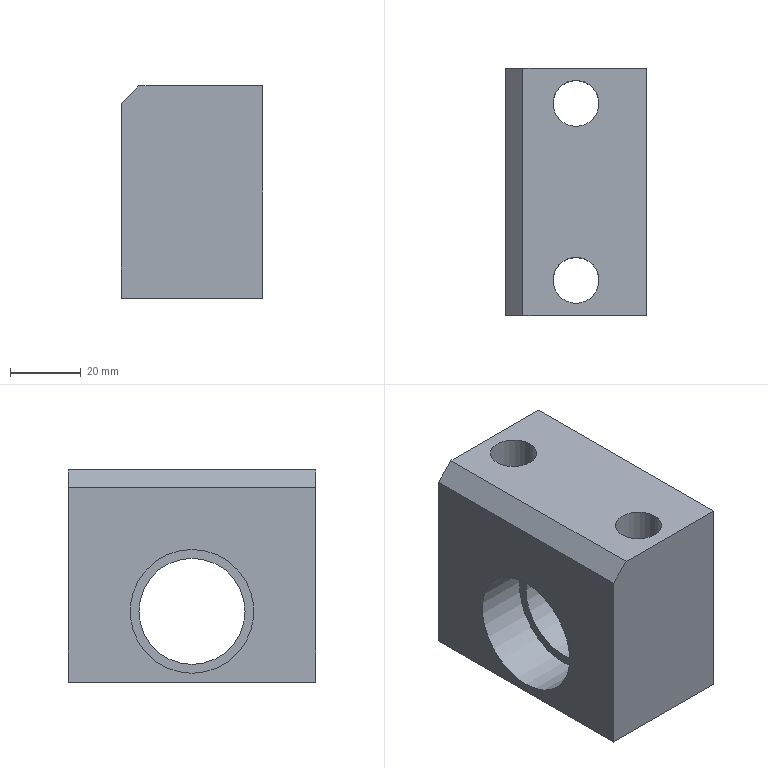Part | NX | features solid 2 | 1 solid | 12 faces | box 40 x 70 x 60 mm | volume 119094 mm3 | plane 8 | cylinder 4 | commonest cylinder face diameters 13 x2 30 x1 35 x1
STEP:
#1=CARTESIAN_POINT('',(-363.5,145.,200.));
#2=VERTEX_POINT('',#1);
#3=CARTESIAN_POINT('',(-370.,145.,200.));
#4=DIRECTION('',(0.,0.,1.));
#5=DIRECTION('',(1.,0.,0.));
#6=AXIS2_PLACEMENT_3D('',#3,#4,#5);
#7=CIRCLE('',#6,6.5);
#8=EDGE_CURVE('',#2,#2,#7,.F.);
#9=ORIENTED_EDGE('',*,*,#8,.T.);
#10=EDGE_LOOP('',(#9));
#11=FACE_BOUND('',#10,.T.);
#12=CARTESIAN_POINT('',(-363.5,195.,200.));
#13=VERTEX_POINT('',#12);
#14=CARTESIAN_POINT('',(-370.,195.,200.));
#15=DIRECTION('',(0.,0.,1.));
#16=DIRECTION('',(1.,0.,0.));
#17=AXIS2_PLACEMENT_3D('',#14,#15,#16);
#18=CIRCLE('',#17,6.5);
#19=EDGE_CURVE('',#13,#13,#18,.F.);
#20=ORIENTED_EDGE('',*,*,#19,.T.);
#21=EDGE_LOOP('',(#20));
#22=FACE_BOUND('',#21,.T.);
#23=CARTESIAN_POINT('',(-350.,205.,200.));
#24=VERTEX_POINT('',#23);
#25=CARTESIAN_POINT('',(-385.,205.,200.));
#26=VERTEX_POINT('',#25);
#27=CARTESIAN_POINT('',(-350.,205.,200.));
#28=DIRECTION('',(1.,0.,0.));
#29=VECTOR('',#28,1000.);
#30=LINE('',#27,#29);
#31=EDGE_CURVE('',#24,#26,#30,.F.);
#32=ORIENTED_EDGE('',*,*,#31,.T.);
#33=CARTESIAN_POINT('',(-385.,135.,200.));
#34=VERTEX_POINT('',#33);
#35=CARTESIAN_POINT('',(-385.,205.,200.));
#36=DIRECTION('',(0.,1.,0.));
#37=VECTOR('',#36,1000.);
#38=LINE('',#35,#37);
#39=EDGE_CURVE('',#26,#34,#38,.F.);
#40=ORIENTED_EDGE('',*,*,#39,.T.);
#41=CARTESIAN_POINT('',(-350.,135.,200.));
#42=VERTEX_POINT('',#41);
#43=CARTESIAN_POINT('',(-350.,135.,200.));
#44=DIRECTION('',(1.,0.,0.));
#45=VECTOR('',#44,1000.);
#46=LINE('',#43,#45);
#47=EDGE_CURVE('',#42,#34,#46,.F.);
#48=ORIENTED_EDGE('',*,*,#47,.F.);
#49=CARTESIAN_POINT('',(-350.,205.,200.));
#50=DIRECTION('',(0.,-1.,0.));
#51=VECTOR('',#50,1000.);
#52=LINE('',#49,#51);
#53=EDGE_CURVE('',#24,#42,#52,.T.);
#54=ORIENTED_EDGE('',*,*,#53,.F.);
#55=EDGE_LOOP('',(#32,#40,#48,#54));
#56=FACE_BOUND('',#55,.T.);
#57=CARTESIAN_POINT('',(-350.,205.,200.));
#58=DIRECTION('',(0.,0.,1.));
#59=DIRECTION('',(0.,-1.,0.));
#60=AXIS2_PLACEMENT_3D('',#57,#58,#59);
#61=PLANE('',#60);
#62=ADVANCED_FACE('',(#11,#22,#56),#61,.T.);
#63=ORIENTED_EDGE('',*,*,#47,.T.);
#64=CARTESIAN_POINT('',(-390.,135.,195.));
#65=VERTEX_POINT('',#64);
#66=CARTESIAN_POINT('',(-385.,135.,200.));
#67=DIRECTION('',(0.7071,0.,0.7071));
#68=VECTOR('',#67,1000.);
#69=LINE('',#66,#68);
#70=EDGE_CURVE('',#34,#65,#69,.F.);
#71=ORIENTED_EDGE('',*,*,#70,.T.);
#72=CARTESIAN_POINT('',(-390.,135.,140.));
#73=VERTEX_POINT('',#72);
#74=CARTESIAN_POINT('',(-390.,135.,200.));
#75=DIRECTION('',(0.,0.,-1.));
#76=VECTOR('',#75,1000.);
#77=LINE('',#74,#76);
#78=EDGE_CURVE('',#65,#73,#77,.T.);
#79=ORIENTED_EDGE('',*,*,#78,.T.);
#80=CARTESIAN_POINT('',(-350.,135.,140.));
#81=VERTEX_POINT('',#80);
#82=CARTESIAN_POINT('',(-350.,135.,140.));
#83=DIRECTION('',(1.,0.,0.));
#84=VECTOR('',#83,1000.);
#85=LINE('',#82,#84);
#86=EDGE_CURVE('',#81,#73,#85,.F.);
#87=ORIENTED_EDGE('',*,*,#86,.F.);
#88=CARTESIAN_POINT('',(-350.,135.,200.));
#89=DIRECTION('',(0.,0.,-1.));
#90=VECTOR('',#89,1000.);
#91=LINE('',#88,#90);
#92=EDGE_CURVE('',#42,#81,#91,.T.);
#93=ORIENTED_EDGE('',*,*,#92,.F.);
#94=EDGE_LOOP('',(#63,#71,#79,#87,#93));
#95=FACE_BOUND('',#94,.T.);
#96=CARTESIAN_POINT('',(-350.,135.,200.));
#97=DIRECTION('',(0.,-1.,0.));
#98=DIRECTION('',(0.,0.,-1.));
#99=AXIS2_PLACEMENT_3D('',#96,#97,#98);
#100=PLANE('',#99);
#101=ADVANCED_FACE('',(#95),#100,.T.);
#102=CARTESIAN_POINT('',(-363.5,145.,140.));
#103=VERTEX_POINT('',#102);
#104=CARTESIAN_POINT('',(-370.,145.,140.));
#105=DIRECTION('',(0.,0.,1.));
#106=DIRECTION('',(1.,0.,0.));
#107=AXIS2_PLACEMENT_3D('',#104,#105,#106);
#108=CIRCLE('',#107,6.5);
#109=EDGE_CURVE('',#103,#103,#108,.T.);
#110=ORIENTED_EDGE('',*,*,#109,.T.);
#111=EDGE_LOOP('',(#110));
#112=FACE_BOUND('',#111,.T.);
#113=CARTESIAN_POINT('',(-363.5,195.,140.));
#114=VERTEX_POINT('',#113);
#115=CARTESIAN_POINT('',(-370.,195.,140.));
#116=DIRECTION('',(0.,0.,1.));
#117=DIRECTION('',(1.,0.,0.));
#118=AXIS2_PLACEMENT_3D('',#115,#116,#117);
#119=CIRCLE('',#118,6.5);
#120=EDGE_CURVE('',#114,#114,#119,.T.);
#121=ORIENTED_EDGE('',*,*,#120,.T.);
#122=EDGE_LOOP('',(#121));
#123=FACE_BOUND('',#122,.T.);
#124=ORIENTED_EDGE('',*,*,#86,.T.);
#125=CARTESIAN_POINT('',(-390.,205.,140.));
#126=VERTEX_POINT('',#125);
#127=CARTESIAN_POINT('',(-390.,205.,140.));
#128=DIRECTION('',(0.,1.,0.));
#129=VECTOR('',#128,1000.);
#130=LINE('',#127,#129);
#131=EDGE_CURVE('',#126,#73,#130,.F.);
#132=ORIENTED_EDGE('',*,*,#131,.F.);
#133=CARTESIAN_POINT('',(-350.,205.,140.));
#134=VERTEX_POINT('',#133);
#135=CARTESIAN_POINT('',(-350.,205.,140.));
#136=DIRECTION('',(1.,0.,0.));
#137=VECTOR('',#136,1000.);
#138=LINE('',#135,#137);
#139=EDGE_CURVE('',#134,#126,#138,.F.);
#140=ORIENTED_EDGE('',*,*,#139,.F.);
#141=CARTESIAN_POINT('',(-350.,205.,140.));
#142=DIRECTION('',(0.,-1.,0.));
#143=VECTOR('',#142,1000.);
#144=LINE('',#141,#143);
#145=EDGE_CURVE('',#134,#81,#144,.T.);
#146=ORIENTED_EDGE('',*,*,#145,.T.);
#147=EDGE_LOOP('',(#124,#132,#140,#146));
#148=FACE_BOUND('',#147,.T.);
#149=CARTESIAN_POINT('',(-350.,205.,140.));
#150=DIRECTION('',(0.,0.,1.));
#151=DIRECTION('',(0.,-1.,0.));
#152=AXIS2_PLACEMENT_3D('',#149,#150,#151);
#153=PLANE('',#152);
#154=ADVANCED_FACE('',(#112,#123,#148),#153,.F.);
#155=CARTESIAN_POINT('',(-390.,205.,195.));
#156=VERTEX_POINT('',#155);
#157=CARTESIAN_POINT('',(-390.,205.,200.));
#158=DIRECTION('',(0.,0.,-1.));
#159=VECTOR('',#158,1000.);
#160=LINE('',#157,#159);
#161=EDGE_CURVE('',#156,#126,#160,.T.);
#162=ORIENTED_EDGE('',*,*,#161,.F.);
#163=CARTESIAN_POINT('',(-385.,205.,200.));
#164=DIRECTION('',(0.7071,0.,0.7071));
#165=VECTOR('',#164,1000.);
#166=LINE('',#163,#165);
#167=EDGE_CURVE('',#156,#26,#166,.T.);
#168=ORIENTED_EDGE('',*,*,#167,.T.);
#169=ORIENTED_EDGE('',*,*,#31,.F.);
#170=CARTESIAN_POINT('',(-350.,205.,200.));
#171=DIRECTION('',(0.,0.,-1.));
#172=VECTOR('',#171,1000.);
#173=LINE('',#170,#172);
#174=EDGE_CURVE('',#24,#134,#173,.T.);
#175=ORIENTED_EDGE('',*,*,#174,.T.);
#176=ORIENTED_EDGE('',*,*,#139,.T.);
#177=EDGE_LOOP('',(#162,#168,#169,#175,#176));
#178=FACE_BOUND('',#177,.T.);
#179=CARTESIAN_POINT('',(-350.,205.,200.));
#180=DIRECTION('',(0.,-1.,0.));
#181=DIRECTION('',(0.,0.,-1.));
#182=AXIS2_PLACEMENT_3D('',#179,#180,#181);
#183=PLANE('',#182);
#184=ADVANCED_FACE('',(#178),#183,.F.);
#185=CARTESIAN_POINT('',(-390.,170.,142.5));
#186=VERTEX_POINT('',#185);
#187=CARTESIAN_POINT('',(-390.,170.,160.));
#188=DIRECTION('',(1.,0.,0.));
#189=DIRECTION('',(0.,0.,-1.));
#190=AXIS2_PLACEMENT_3D('',#187,#188,#189);
#191=CIRCLE('',#190,17.5);
#192=EDGE_CURVE('',#186,#186,#191,.T.);
#193=ORIENTED_EDGE('',*,*,#192,.T.);
#194=EDGE_LOOP('',(#193));
#195=FACE_BOUND('',#194,.T.);
#196=ORIENTED_EDGE('',*,*,#78,.F.);
#197=CARTESIAN_POINT('',(-390.,205.,195.));
#198=DIRECTION('',(0.,1.,0.));
#199=VECTOR('',#198,1000.);
#200=LINE('',#197,#199);
#201=EDGE_CURVE('',#65,#156,#200,.T.);
#202=ORIENTED_EDGE('',*,*,#201,.T.);
#203=ORIENTED_EDGE('',*,*,#161,.T.);
#204=ORIENTED_EDGE('',*,*,#131,.T.);
#205=EDGE_LOOP('',(#196,#202,#203,#204));
#206=FACE_BOUND('',#205,.T.);
#207=CARTESIAN_POINT('',(-390.,205.,200.));
#208=DIRECTION('',(1.,0.,0.));
#209=DIRECTION('',(0.,0.,-1.));
#210=AXIS2_PLACEMENT_3D('',#207,#208,#209);
#211=PLANE('',#210);
#212=ADVANCED_FACE('',(#195,#206),#211,.F.);
#213=CARTESIAN_POINT('',(-350.,170.,145.));
#214=VERTEX_POINT('',#213);
#215=CARTESIAN_POINT('',(-350.,170.,160.));
#216=DIRECTION('',(1.,0.,0.));
#217=DIRECTION('',(0.,0.,-1.));
#218=AXIS2_PLACEMENT_3D('',#215,#216,#217);
#219=CIRCLE('',#218,15.);
#220=EDGE_CURVE('',#214,#214,#219,.T.);
#221=ORIENTED_EDGE('',*,*,#220,.F.);
#222=EDGE_LOOP('',(#221));
#223=FACE_BOUND('',#222,.T.);
#224=ORIENTED_EDGE('',*,*,#145,.F.);
#225=ORIENTED_EDGE('',*,*,#174,.F.);
#226=ORIENTED_EDGE('',*,*,#53,.T.);
#227=ORIENTED_EDGE('',*,*,#92,.T.);
#228=EDGE_LOOP('',(#224,#225,#226,#227));
#229=FACE_BOUND('',#228,.T.);
#230=CARTESIAN_POINT('',(-350.,205.,200.));
#231=DIRECTION('',(1.,0.,0.));
#232=DIRECTION('',(0.,0.,-1.));
#233=AXIS2_PLACEMENT_3D('',#230,#231,#232);
#234=PLANE('',#233);
#235=ADVANCED_FACE('',(#223,#229),#234,.T.);
#236=ORIENTED_EDGE('',*,*,#120,.F.);
#237=EDGE_LOOP('',(#236));
#238=FACE_BOUND('',#237,.T.);
#239=ORIENTED_EDGE('',*,*,#19,.F.);
#240=EDGE_LOOP('',(#239));
#241=FACE_BOUND('',#240,.T.);
#242=CARTESIAN_POINT('',(-370.,195.,140.));
#243=DIRECTION('',(0.,0.,1.));
#244=DIRECTION('',(1.,0.,0.));
#245=AXIS2_PLACEMENT_3D('',#242,#243,#244);
#246=CYLINDRICAL_SURFACE('',#245,6.5);
#247=ADVANCED_FACE('',(#238,#241),#246,.F.);
#248=ORIENTED_EDGE('',*,*,#109,.F.);
#249=EDGE_LOOP('',(#248));
#250=FACE_BOUND('',#249,.T.);
#251=ORIENTED_EDGE('',*,*,#8,.F.);
#252=EDGE_LOOP('',(#251));
#253=FACE_BOUND('',#252,.T.);
#254=CARTESIAN_POINT('',(-370.,145.,140.));
#255=DIRECTION('',(0.,0.,1.));
#256=DIRECTION('',(1.,0.,0.));
#257=AXIS2_PLACEMENT_3D('',#254,#255,#256);
#258=CYLINDRICAL_SURFACE('',#257,6.5);
#259=ADVANCED_FACE('',(#250,#253),#258,.F.);
#260=ORIENTED_EDGE('',*,*,#220,.T.);
#261=EDGE_LOOP('',(#260));
#262=FACE_BOUND('',#261,.T.);
#263=CARTESIAN_POINT('',(-375.,170.,145.));
#264=VERTEX_POINT('',#263);
#265=CARTESIAN_POINT('',(-375.,170.,160.));
#266=DIRECTION('',(1.,0.,0.));
#267=DIRECTION('',(0.,0.,-1.));
#268=AXIS2_PLACEMENT_3D('',#265,#266,#267);
#269=CIRCLE('',#268,15.);
#270=EDGE_CURVE('',#264,#264,#269,.T.);
#271=ORIENTED_EDGE('',*,*,#270,.F.);
#272=EDGE_LOOP('',(#271));
#273=FACE_BOUND('',#272,.T.);
#274=CARTESIAN_POINT('',(-290.,170.,160.));
#275=DIRECTION('',(1.,0.,0.));
#276=DIRECTION('',(0.,0.,-1.));
#277=AXIS2_PLACEMENT_3D('',#274,#275,#276);
#278=CYLINDRICAL_SURFACE('',#277,15.);
#279=ADVANCED_FACE('',(#262,#273),#278,.F.);
#280=ORIENTED_EDGE('',*,*,#270,.T.);
#281=EDGE_LOOP('',(#280));
#282=FACE_BOUND('',#281,.T.);
#283=CARTESIAN_POINT('',(-375.,170.,142.5));
#284=VERTEX_POINT('',#283);
#285=CARTESIAN_POINT('',(-375.,170.,160.));
#286=DIRECTION('',(1.,0.,0.));
#287=DIRECTION('',(0.,0.,-1.));
#288=AXIS2_PLACEMENT_3D('',#285,#286,#287);
#289=CIRCLE('',#288,17.5);
#290=EDGE_CURVE('',#284,#284,#289,.T.);
#291=ORIENTED_EDGE('',*,*,#290,.F.);
#292=EDGE_LOOP('',(#291));
#293=FACE_BOUND('',#292,.T.);
#294=CARTESIAN_POINT('',(-375.,170.,160.));
#295=DIRECTION('',(1.,0.,0.));
#296=DIRECTION('',(0.,0.,-1.));
#297=AXIS2_PLACEMENT_3D('',#294,#295,#296);
#298=PLANE('',#297);
#299=ADVANCED_FACE('',(#282,#293),#298,.F.);
#300=ORIENTED_EDGE('',*,*,#290,.T.);
#301=EDGE_LOOP('',(#300));
#302=FACE_BOUND('',#301,.T.);
#303=ORIENTED_EDGE('',*,*,#192,.F.);
#304=EDGE_LOOP('',(#303));
#305=FACE_BOUND('',#304,.T.);
#306=CARTESIAN_POINT('',(-390.,170.,160.));
#307=DIRECTION('',(1.,0.,0.));
#308=DIRECTION('',(0.,0.,-1.));
#309=AXIS2_PLACEMENT_3D('',#306,#307,#308);
#310=CYLINDRICAL_SURFACE('',#309,17.5);
#311=ADVANCED_FACE('',(#302,#305),#310,.F.);
#312=ORIENTED_EDGE('',*,*,#167,.F.);
#313=ORIENTED_EDGE('',*,*,#201,.F.);
#314=ORIENTED_EDGE('',*,*,#70,.F.);
#315=ORIENTED_EDGE('',*,*,#39,.F.);
#316=EDGE_LOOP('',(#312,#313,#314,#315));
#317=FACE_BOUND('',#316,.T.);
#318=CARTESIAN_POINT('',(-385.,205.,200.));
#319=DIRECTION('',(-0.7071,0.,0.7071));
#320=DIRECTION('',(0.7071,0.,0.7071));
#321=AXIS2_PLACEMENT_3D('',#318,#319,#320);
#322=PLANE('',#321);
#323=ADVANCED_FACE('',(#317),#322,.T.);
#324=CLOSED_SHELL('',(#62,#101,#154,#184,#212,#235,#247,#259,#279,#299,#311,#323));
#325=MANIFOLD_SOLID_BREP('',#324);
#326=(LENGTH_UNIT()NAMED_UNIT(*)SI_UNIT(.MILLI.,.METRE.));
#327=UNCERTAINTY_MEASURE_WITH_UNIT(LENGTH_MEASURE(0.00001),#326,'','');
#328=(NAMED_UNIT(*)PLANE_ANGLE_UNIT()SI_UNIT($,.RADIAN.));
#329=(NAMED_UNIT(*)SI_UNIT($,.STERADIAN.)SOLID_ANGLE_UNIT());
#330=(GEOMETRIC_REPRESENTATION_CONTEXT(3)GLOBAL_UNCERTAINTY_ASSIGNED_CONTEXT((#327))GLOBAL_UNIT_ASSIGNED_CONTEXT((#326,#328,#329))REPRESENTATION_CONTEXT('',''));
#331=ADVANCED_BREP_SHAPE_REPRESENTATION('',(#325),#330);